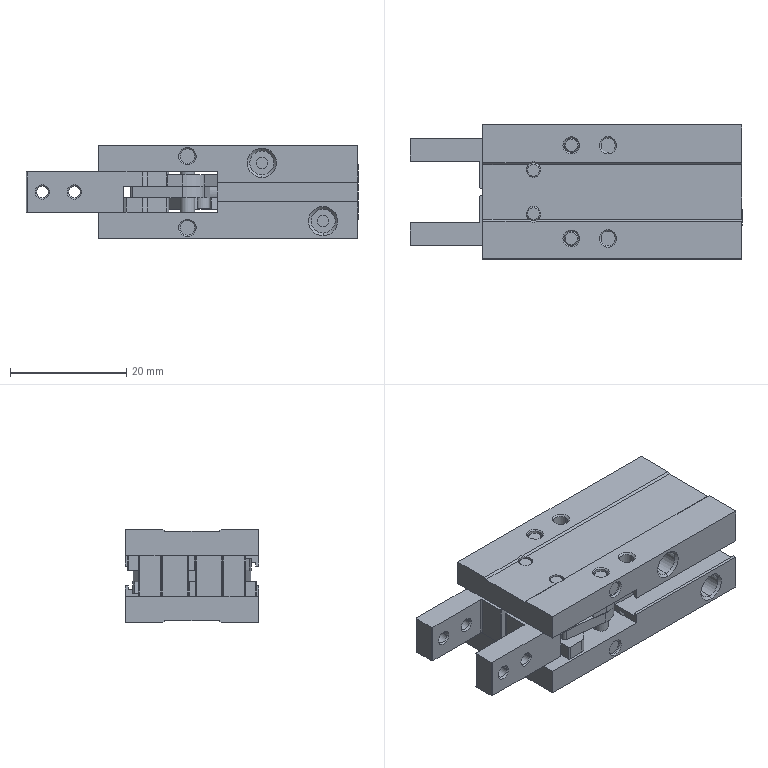Part | SolidWorks | 2 solids | 372 faces | box 57 x 23 x 16 mm | volume 13388 mm3 | plane 157 | cylinder 135 | cone 80 | commonest cylinder face diameters 2.5 x54 2.459 x16 2 x14 0.4 x12 2.013 x8 2.52 x6